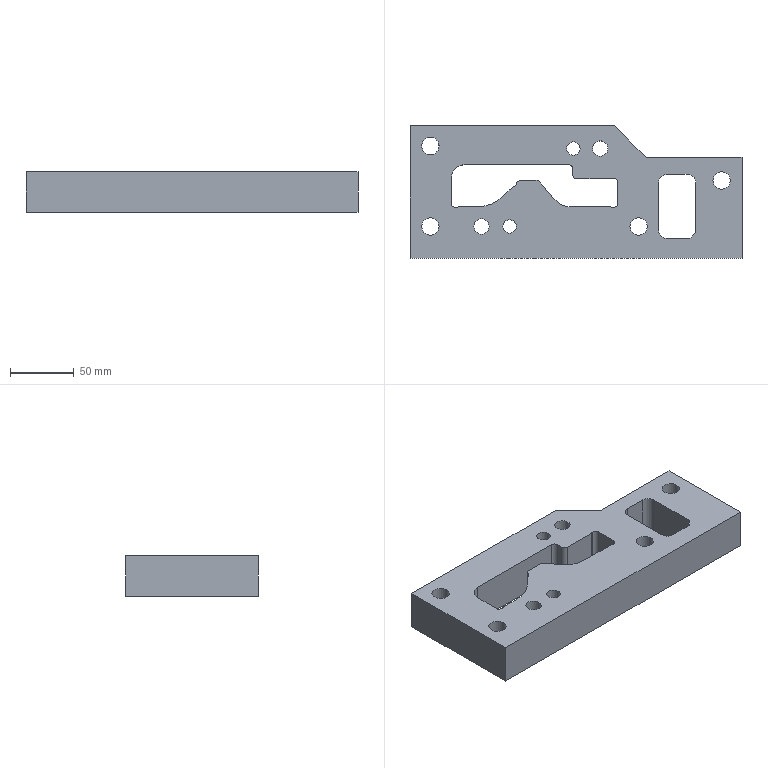Part | STEP file | lll_id110_x_t | 1 solid | 57 faces | box 260 x 104 x 32 mm | volume 608123 mm3 | cylinder 30 | plane 27 | commonest cylinder face diameters 6 x8 12 x5 13.509 x4 20.008 x4 8 x3 10.505 x2